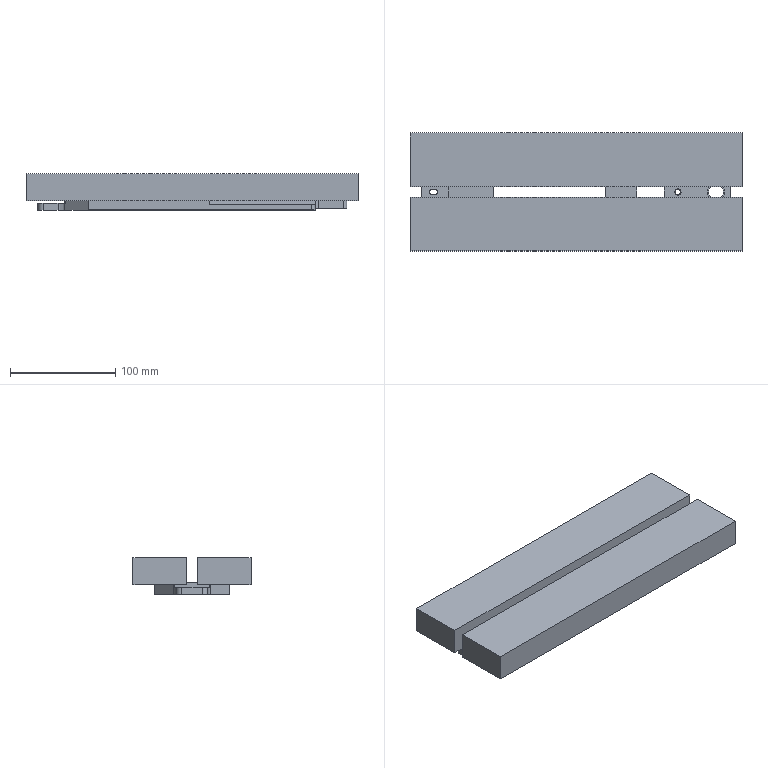CAM job | NX | 3-axis milling, drilling | part box 315 x 112 x 34.85 mm
Tools:
number,name,description,diameter,corner_radius,flute_length,length,flutes
1,D100面刀,Milling Tool-5 Parameters,100.0,0.0,50.0,75.0,2
2,D12_ROUGH,Milling Tool-5 Parameters,12.0,0.0,50.0,75.0,2
3,D4开粗,Milling Tool-5 Parameters,4.0,0.0,50.0,75.0,2
4,D8点钻,Drilling Tool,8.0,0.0,35.0,50.0,2
5,D3.4_DRILL,Drilling Tool,3.4,0.0,35.0,50.0,2
6,D4.5_DRILL,Drilling Tool,4.5,0.0,35.0,50.0,2
7,D2.3_DRILL,Drilling Tool,2.3,0.0,35.0,50.0,2
8,M2.5,Drilling Tool,2.5,0.0,35.0,50.0,2
9,D6精光,Milling Tool-5 Parameters,6.0,0.0,50.0,75.0,2
10,D4精光,Milling Tool-5 Parameters,4.0,0.0,50.0,75.0,2
11,D2_FINISH,Milling Tool-5 Parameters,2.0,0.0,50.0,75.0,2
12,D3倒角刀,Milling Tool-5 Parameters,3.0,0.0,50.0,75.0,2
0,5.5_DRILL,Milling Tool-5 Parameters,5.5,0.0,50.0,75.0,2
Operations:
program,operation,operation_type,tool,method,geometry_group,spindle_rpm,surface_speed,feed_per_tooth,feed_cut,feed_plunge,cut_length_mm,path_length_mm,cut_time_min,machine_time_min
G54,PLANAR_MILL,PlanarMilling,D100面刀,METHOD,54,3500.0,879.0,0.1143,800.0,100.0,431.0,465.0,0.5388,0.5422
G54,ADAPTIVE_MILLING,CavityMilling,D12_ROUGH,METHOD,54,6500.0,245.0,0.2308,3000.0,100.0,17637.071,18838.246,5.81,5.931
G54,ADAPTIVE_MILLING_COPY,CavityMilling,D4开粗,METHOD,54,6500.0,81.0,0.1538,2000.0,100.0,3112.387,4319.53,1.55,1.671
G54,DRILLING,Operation,D8点钻,METHOD,54,2500.0,62.0,0.04,200.0,0.0,18.8,144.31,0.094,0.1066
G54,DRILLING_COPY,Operation,D8点钻,METHOD,54,2500.0,62.0,0.04,200.0,0.0,11.2,102.084,0.056,0.0651
G54,DRILLING_COPY_COPY_1,Operation,D8点钻,METHOD,54,2500.0,62.0,0.04,200.0,0.0,5.8,51.6,0.029,0.0336
G54,DRILLING_COPY_COPY,Operation,D8点钻,METHOD,54,2500.0,62.0,0.04,200.0,0.0,16.8,313.78,0.084,0.1137
G54,DRILLING_COPY_1,Operation,D3.4_DRILL,METHOD,54,2500.0,26.0,0.04,200.0,0.0,64.0,234.71,0.32,0.3371
G54,DRILLING_COPY_COPY_2,Operation,D4.5_DRILL,METHOD,54,2500.0,26.0,0.04,200.0,0.0,32.0,125.525,0.16,0.1694
G54,DRILLING_COPY_COPY_2_COPY,Operation,5.5_DRILL,METHOD,54,2500.0,26.0,0.04,200.0,0.0,16.0,72.0,0.08,0.0856
G54,DRILLING_COPY_COPY_COPY,Operation,D2.3_DRILL,METHOD,54,2500.0,26.0,0.04,200.0,0.0,64.0,408.18,0.32,0.3544
G54,DRILLING_COPY_COPY_COPY_COPY,Operation,M2.5,METHOD,54,300.0,2.0,0.0008,0.45,0.0,56.0,392.18,124.444,124.478
G54,PLANAR_MILL_7_COPY_1,PlanarMilling,D4精光,METHOD,54,4500.0,56.0,0.0667,600.0,100.0,167.721,218.171,0.2795,0.2846
G54,PLANAR_MILL_1,PlanarMilling,D6精光,METHOD,54,5500.0,103.0,0.0909,1000.0,100.0,1443.4,1501.1,1.443,1.449
G54,PLANAR_MILL_1_COPY,PlanarMilling,D6精光,METHOD,54,5500.0,103.0,0.0091,100.0,100.0,66.718,124.418,0.6672,0.673
G54,PLANAR_MILL_1_COPY_COPY_1,PlanarMilling,D6精光,METHOD,54,5500.0,103.0,0.0909,600.0,100.0,286.288,343.988,0.4771,0.4829
G54,PLANAR_MILL_1_COPY_COPY,PlanarMilling,D6精光,METHOD,54,5500.0,103.0,0.0091,100.0,100.0,82.197,124.197,0.822,0.8262
G54,FLOOR_WALL,VolumeBased25DMillingOperation,D6精光,METHOD,54,5500.0,103.0,0.0909,600.0,100.0,535.494,705.5,0.8925,0.9095
G54,PLANAR_MILL_6,PlanarMilling,D6精光,METHOD,54,5500.0,103.0,0.0727,800.0,100.0,233.279,361.362,0.2916,0.3044
G54,FLOOR_WALL_1,VolumeBased25DMillingOperation,D6精光,METHOD,54,5500.0,103.0,0.0909,600.0,100.0,202.723,244.723,0.3379,0.3421
G54,PLANAR_MILL_6_COPY,PlanarMilling,D6精光,METHOD,54,5500.0,103.0,0.0727,800.0,100.0,54.828,96.818,0.0685,0.0727
G54,PLANAR_MILL_1_COPY_1,PlanarMilling,D6精光,METHOD,54,5500.0,103.0,0.0909,1000.0,100.0,116.489,272.674,0.1165,0.1321
G54,PLANAR_MILL_7,PlanarMilling,D4精光,METHOD,54,4500.0,56.0,0.0667,600.0,100.0,158.606,209.556,0.2643,0.2694
G54,PLANAR_MILL_7_COPY,PlanarMilling,D4精光,METHOD,54,5500.0,69.0,0.0073,80.0,100.0,14.14,70.24,0.1767,0.1824
G54,PLANAR_MILL_2,PlanarMilling,D4精光,METHOD,54,4500.0,56.0,0.0667,600.0,100.0,349.077,396.077,0.5818,0.5865
G54,PLANAR_MILL_2_COPY,PlanarMilling,D4精光,METHOD,54,4500.0,56.0,0.0889,800.0,100.0,109.742,156.742,0.1372,0.1419
G54,PLANAR_MILL_2_COPY_COPY,PlanarMilling,D4精光,METHOD,54,4500.0,56.0,0.0889,600.0,100.0,134.026,192.726,0.2234,0.2292
G54,PLANAR_MILL_2_COPY_COPY_1,PlanarMilling,D4精光,METHOD,54,4500.0,56.0,0.0889,800.0,100.0,109.742,156.742,0.1372,0.1419
G54,PLANAR_MILL_3,PlanarMilling,D2_FINISH,METHOD,54,5000.0,31.0,0.1,1000.0,100.0,744.84,1010.134,0.7448,0.7714
G54,PLANAR_MILL_3_COPY,PlanarMilling,D2_FINISH,METHOD,54,4500.0,28.0,0.0333,300.0,100.0,61.706,317.388,0.2057,0.2313
G54,PLANAR_MILL_4_COPY_1,PlanarMilling,D2_FINISH,METHOD,54,4500.0,28.0,0.1111,1000.0,100.0,152.736,201.686,0.1527,0.1576
G54,PLANAR_MILL_4,PlanarMilling,D2_FINISH,METHOD,54,4500.0,28.0,0.1111,1000.0,100.0,155.563,204.513,0.1556,0.1605
G54,PLANAR_MILL_4_COPY,PlanarMilling,D2_FINISH,METHOD,54,4500.0,28.0,0.0333,300.0,100.0,21.71,67.61,0.0724,0.077
G54,PLANAR_MILL_5,PlanarMilling,D3倒角刀,METHOD,54,4500.0,42.0,0.1111,1000.0,100.0,629.649,667.649,0.6296,0.6334
G54,PLANAR_MILL_5_COPY,PlanarMilling,D3倒角刀,METHOD,54,4500.0,42.0,0.1111,1000.0,100.0,464.651,746.594,0.4647,0.4928
G54,PLANAR_MILL_5_COPY_1,PlanarMilling,D3倒角刀,METHOD,54,4500.0,42.0,0.1111,1000.0,100.0,93.044,204.894,0.093,0.1042
G54,PLANAR_MILL_5_COPY_2,PlanarMilling,D3倒角刀,METHOD,54,4500.0,42.0,0.1111,1000.0,100.0,235.696,407.943,0.2357,0.2529
G54,PLANAR_MILL_5_COPY_3,PlanarMilling,D3倒角刀,METHOD,54,4500.0,42.0,0.1111,1000.0,100.0,123.326,458.69,0.1233,0.1569
G54,PLANAR_MILL_5_COPY_2_COPY,PlanarMilling,D3倒角刀,METHOD,54,4500.0,42.0,0.1111,1000.0,100.0,45.043,91.043,0.045,0.0496
G55,PLANAR_MILL_8,PlanarMilling,D100面刀,METHOD,G55,4000.0,1256.0,0.125,1000.0,100.0,1724.0,3122.8,1.724,1.864
G55,PLANAR_MILL_8_COPY,PlanarMilling,D100面刀,METHOD,G55,4000.0,1256.0,0.1,800.0,100.0,431.0,465.0,0.5388,0.5422
G55,PLANAR_MILL_9,PlanarMilling,D4开粗,METHOD,G55,4500.0,56.0,0.1111,1000.0,100.0,152.051,196.801,0.1521,0.1565
G55,PLANAR_MILL_10,PlanarMilling,D4开粗,METHOD,G55,4500.0,56.0,0.1111,1000.0,100.0,305.672,429.228,0.3057,0.318
G55,PLANAR_MILL_11,PlanarMilling,D4开粗,METHOD,G55,4500.0,56.0,0.1111,1000.0,100.0,434.175,543.529,0.4342,0.4451
G55,PLANAR_MILL_10_COPY,PlanarMilling,D4精光,METHOD,G55,3500.0,43.0,0.0571,400.0,100.0,56.458,180.251,0.1411,0.1535
G55,PLANAR_MILL_11_COPY,PlanarMilling,D4精光,METHOD,G55,3500.0,56.0,0.0889,400.0,100.0,116.544,201.016,0.2914,0.2998
G55,PLANAR_MILL_9_COPY_1,PlanarMilling,D4精光,METHOD,G55,3500.0,56.0,0.0889,400.0,100.0,30.106,74.706,0.0753,0.0797
G55,FLOOR_WALL_2,VolumeBased25DMillingOperation,D6精光,METHOD,55,4500.0,84.0,0.1111,1000.0,100.0,403.65,492.274,0.4036,0.4125
G55,FLOOR_WALL_2_COPY,VolumeBased25DMillingOperation,D6精光,METHOD,55,3500.0,65.0,0.1143,800.0,100.0,202.225,239.925,0.2528,0.2566
G55,PLANAR_MILL_14,PlanarMilling,D6精光,METHOD,55,3500.0,65.0,0.1143,800.0,100.0,43.283,81.083,0.0541,0.0579
G55,PLANAR_MILL_13,PlanarMilling,D3倒角刀,METHOD,55,4500.0,42.0,0.0889,800.0,100.0,107.509,486.673,0.1344,0.1723
G55,PLANAR_MILL_15,PlanarMilling,D3倒角刀,METHOD,55,4500.0,42.0,0.0889,800.0,100.0,134.931,170.931,0.1687,0.1723
G55,PLANAR_MILL_17,PlanarMilling,D3倒角刀,METHOD,G55,4500.0,42.0,0.0889,800.0,100.0,229.712,514.451,0.2871,0.3156
G55,PLANAR_MILL_19,PlanarMilling,D3倒角刀,METHOD,G55,4500.0,42.0,0.0889,800.0,100.0,88.708,128.408,0.1109,0.1149
G55,PLANAR_MILL_20,PlanarMilling,D3倒角刀,METHOD,G55,4500.0,42.0,0.0889,800.0,100.0,47.043,86.743,0.0588,0.0628
G55,PLANAR_MILL_16,PlanarMilling,D3倒角刀,METHOD,G55,4500.0,42.0,0.0889,800.0,100.0,60.106,285.706,0.0751,0.0977
G55,DRILLING_3,Operation,D8点钻,METHOD,G55,1500.0,37.0,0.0833,250.0,0.0,16.6,313.38,0.0664,0.0961
G55,DRILLING_1,Operation,D8点钻,METHOD,G55,1200.0,30.0,0.0625,150.0,0.0,22.8,156.01,0.152,0.1653
G55,PLANAR_MILL_12,PlanarMilling,D8点钻,METHOD,55,3000.0,75.0,0.1333,800.0,100.0,299.655,336.255,0.3746,0.3782
G55,PLANAR_MILL_18,PlanarMilling,D8点钻,METHOD,G55,3000.0,75.0,0.1333,800.0,100.0,457.2,603.8,0.5715,0.5862
G55,DRILLING_2,Operation,D8点钻,METHOD,G55,2000.0,50.0,0.0375,150.0,0.0,5.6,51.2,0.0373,0.0419
PROGRAM_1,CAVITY_MILL_COPY_COPY,CavityMilling,D4开粗,METHOD,WORKPIECE,6500.0,81.0,0.1538,2000.0,100.0,47928.429,48081.854,23.964,23.98
PROGRAM_1,CAVITY_MILL_COPY_COPY_COPY,CavityMilling,D4开粗,METHOD,WORKPIECE,6500.0,81.0,0.0538,700.0,100.0,5998.318,6105.918,8.569,8.58
PROGRAM_1,CAVITY_MILL_COPY_COPY_COPY_COPY,CavityMilling,D4开粗,METHOD,WORKPIECE,6500.0,81.0,0.0538,700.0,100.0,754.094,900.769,1.077,1.092
XX-CNC1,PLANAR_MILL_10_COPY_1,PlanarMilling,D4开粗,METHOD,MCS_1,4500.0,56.0,0.0333,300.0,100.0,68.678,237.861,0.2289,0.2458
XX-CNC1,DRILLING_1_COPY,Operation,D8点钻,METHOD,MCS_1,1200.0,30.0,0.0625,150.0,0.0,25.6,181.61,0.1707,0.1863
XX-CNC1,PLANAR_MILL_9_COPY,PlanarMilling,D4开粗,METHOD,MCS_1,4500.0,56.0,0.1111,1000.0,100.0,36.38,103.08,0.0364,0.0431